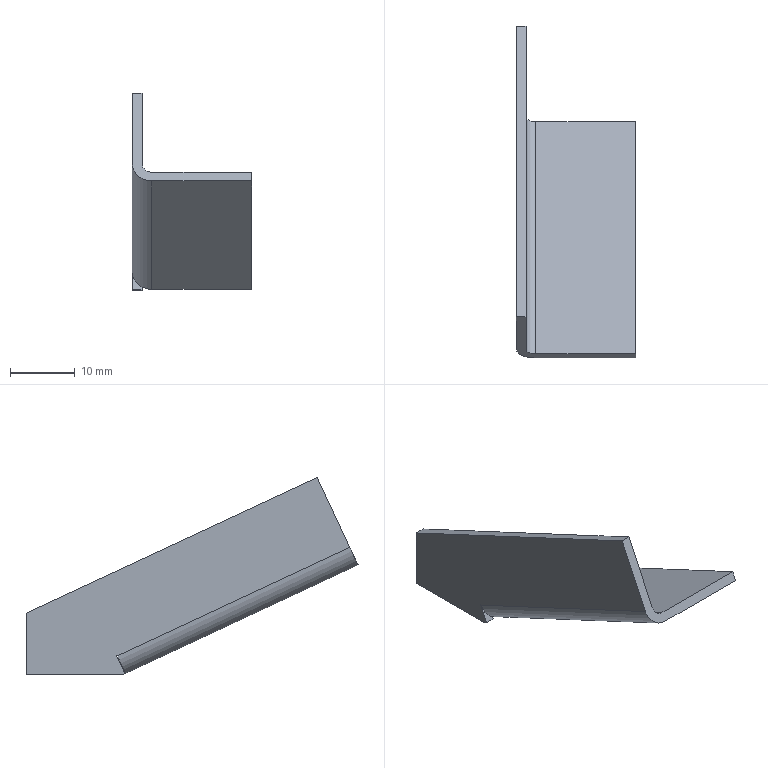Part | NX | features solid 2 | 1 solid | 15 faces | box 18.5 x 51.479 x 30.607 mm | volume 2077 mm3 | plane 13 | cylinder 2 | commonest cylinder face diameters 3 x1 6 x1
STEP:
#1=CARTESIAN_POINT('',(1091.5,-1287.659,323.577));
#2=VERTEX_POINT('',#1);
#3=CARTESIAN_POINT('',(1091.5,-1323.711,340.388));
#4=VERTEX_POINT('',#3);
#5=CARTESIAN_POINT('',(1091.5,-1287.659,323.577));
#6=DIRECTION('',(0.,-0.9063,0.4226));
#7=VECTOR('',#6,1000.);
#8=LINE('',#5,#7);
#9=EDGE_CURVE('',#2,#4,#8,.T.);
#10=ORIENTED_EDGE('',*,*,#9,.T.);
#11=CARTESIAN_POINT('',(1093.,-1324.345,339.028));
#12=VERTEX_POINT('',#11);
#13=CARTESIAN_POINT('',(1093.,-1323.711,340.388));
#14=DIRECTION('',(0.,-0.9063,0.4226));
#15=DIRECTION('',(0.,-0.4226,-0.9063));
#16=AXIS2_PLACEMENT_3D('',#13,#14,#15);
#17=CIRCLE('',#16,1.5);
#18=EDGE_CURVE('',#4,#12,#17,.T.);
#19=ORIENTED_EDGE('',*,*,#18,.T.);
#20=CARTESIAN_POINT('',(1093.,-1288.293,322.217));
#21=VERTEX_POINT('',#20);
#22=CARTESIAN_POINT('',(1093.,-1324.345,339.028));
#23=DIRECTION('',(0.,0.9063,-0.4226));
#24=VECTOR('',#23,1000.);
#25=LINE('',#22,#24);
#26=EDGE_CURVE('',#12,#21,#25,.T.);
#27=ORIENTED_EDGE('',*,*,#26,.T.);
#28=CARTESIAN_POINT('',(1093.,-1287.659,323.577));
#29=DIRECTION('',(0.,0.9063,-0.4226));
#30=DIRECTION('',(0.,-0.4226,-0.9063));
#31=AXIS2_PLACEMENT_3D('',#28,#29,#30);
#32=CIRCLE('',#31,1.5);
#33=EDGE_CURVE('',#21,#2,#32,.T.);
#34=ORIENTED_EDGE('',*,*,#33,.T.);
#35=EDGE_LOOP('',(#10,#19,#27,#34));
#36=FACE_BOUND('',#35,.T.);
#37=CARTESIAN_POINT('',(1093.,-1287.659,323.577));
#38=DIRECTION('',(0.,-0.9063,0.4226));
#39=DIRECTION('',(1.,0.,0.));
#40=AXIS2_PLACEMENT_3D('',#37,#38,#39);
#41=CYLINDRICAL_SURFACE('',#40,1.5);
#42=ADVANCED_FACE('',(#36),#41,.F.);
#43=CARTESIAN_POINT('',(1090.,-1287.659,323.577));
#44=VERTEX_POINT('',#43);
#45=CARTESIAN_POINT('',(1090.,-1323.711,340.388));
#46=VERTEX_POINT('',#45);
#47=CARTESIAN_POINT('',(1090.,-1287.659,323.577));
#48=DIRECTION('',(0.,-0.9063,0.4226));
#49=VECTOR('',#48,1000.);
#50=LINE('',#47,#49);
#51=EDGE_CURVE('',#44,#46,#50,.T.);
#52=ORIENTED_EDGE('',*,*,#51,.F.);
#53=CARTESIAN_POINT('',(1093.,-1288.927,320.858));
#54=VERTEX_POINT('',#53);
#55=CARTESIAN_POINT('',(1093.,-1287.659,323.577));
#56=DIRECTION('',(0.,0.9063,-0.4226));
#57=DIRECTION('',(1.,0.,0.));
#58=AXIS2_PLACEMENT_3D('',#55,#56,#57);
#59=CIRCLE('',#58,3.);
#60=EDGE_CURVE('',#54,#44,#59,.T.);
#61=ORIENTED_EDGE('',*,*,#60,.F.);
#62=CARTESIAN_POINT('',(1093.,-1324.979,337.669));
#63=VERTEX_POINT('',#62);
#64=CARTESIAN_POINT('',(1093.,-1324.979,337.669));
#65=DIRECTION('',(0.,0.9063,-0.4226));
#66=VECTOR('',#65,1000.);
#67=LINE('',#64,#66);
#68=EDGE_CURVE('',#63,#54,#67,.T.);
#69=ORIENTED_EDGE('',*,*,#68,.F.);
#70=CARTESIAN_POINT('',(1093.,-1323.711,340.388));
#71=DIRECTION('',(0.,-0.9063,0.4226));
#72=DIRECTION('',(1.,0.,0.));
#73=AXIS2_PLACEMENT_3D('',#70,#71,#72);
#74=CIRCLE('',#73,3.);
#75=EDGE_CURVE('',#46,#63,#74,.T.);
#76=ORIENTED_EDGE('',*,*,#75,.F.);
#77=EDGE_LOOP('',(#52,#61,#69,#76));
#78=FACE_BOUND('',#77,.T.);
#79=CARTESIAN_POINT('',(1093.,-1287.659,323.577));
#80=DIRECTION('',(0.,-0.9063,0.4226));
#81=DIRECTION('',(1.,0.,0.));
#82=AXIS2_PLACEMENT_3D('',#79,#80,#81);
#83=CYLINDRICAL_SURFACE('',#82,3.);
#84=ADVANCED_FACE('',(#78),#83,.T.);
#85=CARTESIAN_POINT('',(1108.5,-1288.293,322.217));
#86=VERTEX_POINT('',#85);
#87=CARTESIAN_POINT('',(1108.5,-1324.345,339.028));
#88=VERTEX_POINT('',#87);
#89=CARTESIAN_POINT('',(1108.5,-1288.293,322.217));
#90=DIRECTION('',(0.,-0.9063,0.4226));
#91=VECTOR('',#90,1000.);
#92=LINE('',#89,#91);
#93=EDGE_CURVE('',#86,#88,#92,.T.);
#94=ORIENTED_EDGE('',*,*,#93,.T.);
#95=CARTESIAN_POINT('',(1108.5,-1324.979,337.669));
#96=VERTEX_POINT('',#95);
#97=CARTESIAN_POINT('',(1108.5,-1324.979,337.669));
#98=DIRECTION('',(0.,0.4226,0.9063));
#99=VECTOR('',#98,1000.);
#100=LINE('',#97,#99);
#101=EDGE_CURVE('',#96,#88,#100,.T.);
#102=ORIENTED_EDGE('',*,*,#101,.F.);
#103=CARTESIAN_POINT('',(1108.5,-1288.927,320.858));
#104=VERTEX_POINT('',#103);
#105=CARTESIAN_POINT('',(1108.5,-1288.927,320.858));
#106=DIRECTION('',(0.,-0.9063,0.4226));
#107=VECTOR('',#106,1000.);
#108=LINE('',#105,#107);
#109=EDGE_CURVE('',#104,#96,#108,.T.);
#110=ORIENTED_EDGE('',*,*,#109,.F.);
#111=CARTESIAN_POINT('',(1108.5,-1288.927,320.858));
#112=DIRECTION('',(0.,0.4226,0.9063));
#113=VECTOR('',#112,1000.);
#114=LINE('',#111,#113);
#115=EDGE_CURVE('',#104,#86,#114,.T.);
#116=ORIENTED_EDGE('',*,*,#115,.T.);
#117=EDGE_LOOP('',(#94,#102,#110,#116));
#118=FACE_BOUND('',#117,.T.);
#119=CARTESIAN_POINT('',(1108.5,-1288.927,320.858));
#120=DIRECTION('',(-1.,0.,0.));
#121=DIRECTION('',(0.,0.,1.));
#122=AXIS2_PLACEMENT_3D('',#119,#120,#121);
#123=PLANE('',#122);
#124=ADVANCED_FACE('',(#118),#123,.F.);
#125=ORIENTED_EDGE('',*,*,#26,.F.);
#126=CARTESIAN_POINT('',(1091.292,-1324.345,339.028));
#127=DIRECTION('',(-1.,0.,0.));
#128=VECTOR('',#127,1000.);
#129=LINE('',#126,#128);
#130=EDGE_CURVE('',#88,#12,#129,.T.);
#131=ORIENTED_EDGE('',*,*,#130,.F.);
#132=ORIENTED_EDGE('',*,*,#93,.F.);
#133=CARTESIAN_POINT('',(1091.292,-1288.293,322.217));
#134=DIRECTION('',(1.,0.,0.));
#135=VECTOR('',#134,1000.);
#136=LINE('',#133,#135);
#137=EDGE_CURVE('',#21,#86,#136,.T.);
#138=ORIENTED_EDGE('',*,*,#137,.F.);
#139=EDGE_LOOP('',(#125,#131,#132,#138));
#140=FACE_BOUND('',#139,.T.);
#141=CARTESIAN_POINT('',(1110.,-1092.528,230.93));
#142=DIRECTION('',(0.,-0.4226,-0.9063));
#143=DIRECTION('',(0.,-0.9063,0.4226));
#144=AXIS2_PLACEMENT_3D('',#141,#142,#143);
#145=PLANE('',#144);
#146=ADVANCED_FACE('',(#140),#145,.F.);
#147=CARTESIAN_POINT('',(1091.292,-1324.979,337.669));
#148=DIRECTION('',(-1.,0.,0.));
#149=VECTOR('',#148,1000.);
#150=LINE('',#147,#149);
#151=EDGE_CURVE('',#96,#63,#150,.T.);
#152=ORIENTED_EDGE('',*,*,#151,.T.);
#153=ORIENTED_EDGE('',*,*,#68,.T.);
#154=CARTESIAN_POINT('',(1091.292,-1288.927,320.858));
#155=DIRECTION('',(1.,0.,0.));
#156=VECTOR('',#155,1000.);
#157=LINE('',#154,#156);
#158=EDGE_CURVE('',#54,#104,#157,.T.);
#159=ORIENTED_EDGE('',*,*,#158,.T.);
#160=ORIENTED_EDGE('',*,*,#109,.T.);
#161=EDGE_LOOP('',(#152,#153,#159,#160));
#162=FACE_BOUND('',#161,.T.);
#163=CARTESIAN_POINT('',(1110.,-1093.162,229.571));
#164=DIRECTION('',(0.,-0.4226,-0.9063));
#165=DIRECTION('',(0.,-0.9063,0.4226));
#166=AXIS2_PLACEMENT_3D('',#163,#164,#165);
#167=PLANE('',#166);
#168=ADVANCED_FACE('',(#162),#167,.T.);
#169=CARTESIAN_POINT('',(1091.5,-1287.617,323.667));
#170=VERTEX_POINT('',#169);
#171=CARTESIAN_POINT('',(1091.5,-1287.526,323.625));
#172=VERTEX_POINT('',#171);
#173=CARTESIAN_POINT('',(1091.5,-1287.526,323.625));
#174=DIRECTION('',(0.,0.9063,-0.4226));
#175=VECTOR('',#174,1000.);
#176=LINE('',#173,#175);
#177=EDGE_CURVE('',#170,#172,#176,.T.);
#178=ORIENTED_EDGE('',*,*,#177,.F.);
#179=CARTESIAN_POINT('',(1090.,-1287.617,323.667));
#180=VERTEX_POINT('',#179);
#181=CARTESIAN_POINT('',(1090.,-1287.617,323.667));
#182=DIRECTION('',(-1.,0.,0.));
#183=VECTOR('',#182,1000.);
#184=LINE('',#181,#183);
#185=EDGE_CURVE('',#170,#180,#184,.T.);
#186=ORIENTED_EDGE('',*,*,#185,.T.);
#187=CARTESIAN_POINT('',(1090.,-1287.526,323.625));
#188=VERTEX_POINT('',#187);
#189=CARTESIAN_POINT('',(1090.,-1287.526,323.625));
#190=DIRECTION('',(0.,0.9063,-0.4226));
#191=VECTOR('',#190,1000.);
#192=LINE('',#189,#191);
#193=EDGE_CURVE('',#180,#188,#192,.T.);
#194=ORIENTED_EDGE('',*,*,#193,.T.);
#195=CARTESIAN_POINT('',(1090.,-1287.526,323.625));
#196=DIRECTION('',(-1.,0.,0.));
#197=VECTOR('',#196,1000.);
#198=LINE('',#195,#197);
#199=EDGE_CURVE('',#172,#188,#198,.T.);
#200=ORIENTED_EDGE('',*,*,#199,.F.);
#201=EDGE_LOOP('',(#178,#186,#194,#200));
#202=FACE_BOUND('',#201,.T.);
#203=CARTESIAN_POINT('',(1090.,-1287.526,323.625));
#204=DIRECTION('',(0.,0.4226,0.9063));
#205=DIRECTION('',(1.,0.,0.));
#206=AXIS2_PLACEMENT_3D('',#203,#204,#205);
#207=PLANE('',#206);
#208=ADVANCED_FACE('',(#202),#207,.F.);
#209=ORIENTED_EDGE('',*,*,#199,.T.);
#210=CARTESIAN_POINT('',(1090.,-1288.836,320.815));
#211=VERTEX_POINT('',#210);
#212=CARTESIAN_POINT('',(1090.,-1288.836,320.815));
#213=DIRECTION('',(0.,-0.4226,-0.9063));
#214=VECTOR('',#213,1000.);
#215=LINE('',#212,#214);
#216=EDGE_CURVE('',#188,#211,#215,.T.);
#217=ORIENTED_EDGE('',*,*,#216,.T.);
#218=CARTESIAN_POINT('',(1091.5,-1288.836,320.815));
#219=VERTEX_POINT('',#218);
#220=CARTESIAN_POINT('',(1090.,-1288.836,320.815));
#221=DIRECTION('',(-1.,0.,0.));
#222=VECTOR('',#221,1000.);
#223=LINE('',#220,#222);
#224=EDGE_CURVE('',#219,#211,#223,.T.);
#225=ORIENTED_EDGE('',*,*,#224,.F.);
#226=CARTESIAN_POINT('',(1091.5,-1288.836,320.815));
#227=DIRECTION('',(0.,-0.4226,-0.9063));
#228=VECTOR('',#227,1000.);
#229=LINE('',#226,#228);
#230=EDGE_CURVE('',#172,#219,#229,.T.);
#231=ORIENTED_EDGE('',*,*,#230,.F.);
#232=EDGE_LOOP('',(#209,#217,#225,#231));
#233=FACE_BOUND('',#232,.T.);
#234=CARTESIAN_POINT('',(1090.,-1288.836,320.815));
#235=DIRECTION('',(0.,0.9063,-0.4226));
#236=DIRECTION('',(-1.,0.,0.));
#237=AXIS2_PLACEMENT_3D('',#234,#235,#236);
#238=PLANE('',#237);
#239=ADVANCED_FACE('',(#233),#238,.F.);
#240=ORIENTED_EDGE('',*,*,#9,.F.);
#241=CARTESIAN_POINT('',(1091.5,-1288.927,320.858));
#242=DIRECTION('',(0.,0.4226,0.9063));
#243=VECTOR('',#242,1000.);
#244=LINE('',#241,#243);
#245=EDGE_CURVE('',#2,#170,#244,.T.);
#246=ORIENTED_EDGE('',*,*,#245,.T.);
#247=ORIENTED_EDGE('',*,*,#177,.T.);
#248=ORIENTED_EDGE('',*,*,#230,.T.);
#249=CARTESIAN_POINT('',(1091.5,-1288.496,320.657));
#250=VERTEX_POINT('',#249);
#251=CARTESIAN_POINT('',(1091.5,-1324.979,337.669));
#252=DIRECTION('',(0.,0.9063,-0.4226));
#253=VECTOR('',#252,1000.);
#254=LINE('',#251,#253);
#255=EDGE_CURVE('',#219,#250,#254,.T.);
#256=ORIENTED_EDGE('',*,*,#255,.T.);
#257=CARTESIAN_POINT('',(1091.5,-1273.5,320.657));
#258=VERTEX_POINT('',#257);
#259=CARTESIAN_POINT('',(1091.5,-1288.496,320.657));
#260=DIRECTION('',(0.,1.,0.));
#261=VECTOR('',#260,1000.);
#262=LINE('',#259,#261);
#263=EDGE_CURVE('',#250,#258,#262,.T.);
#264=ORIENTED_EDGE('',*,*,#263,.T.);
#265=CARTESIAN_POINT('',(1091.5,-1273.5,330.215));
#266=VERTEX_POINT('',#265);
#267=CARTESIAN_POINT('',(1091.5,-1273.5,320.657));
#268=DIRECTION('',(0.,0.,1.));
#269=VECTOR('',#268,1000.);
#270=LINE('',#267,#269);
#271=EDGE_CURVE('',#258,#266,#270,.T.);
#272=ORIENTED_EDGE('',*,*,#271,.T.);
#273=CARTESIAN_POINT('',(1091.5,-1318.64,351.264));
#274=VERTEX_POINT('',#273);
#275=CARTESIAN_POINT('',(1091.5,-1273.5,330.215));
#276=DIRECTION('',(0.,-0.9063,0.4226));
#277=VECTOR('',#276,1000.);
#278=LINE('',#275,#277);
#279=EDGE_CURVE('',#266,#274,#278,.T.);
#280=ORIENTED_EDGE('',*,*,#279,.T.);
#281=CARTESIAN_POINT('',(1091.5,-1324.979,337.669));
#282=DIRECTION('',(0.,-0.4226,-0.9063));
#283=VECTOR('',#282,1000.);
#284=LINE('',#281,#283);
#285=EDGE_CURVE('',#274,#4,#284,.T.);
#286=ORIENTED_EDGE('',*,*,#285,.T.);
#287=EDGE_LOOP('',(#240,#246,#247,#248,#256,#264,#272,#280,#286));
#288=FACE_BOUND('',#287,.T.);
#289=CARTESIAN_POINT('',(1091.5,-848.5,754.25));
#290=DIRECTION('',(-1.,0.,0.));
#291=DIRECTION('',(0.,0.,1.));
#292=AXIS2_PLACEMENT_3D('',#289,#290,#291);
#293=PLANE('',#292);
#294=ADVANCED_FACE('',(#288),#293,.F.);
#295=CARTESIAN_POINT('',(1090.,-1273.5,330.215));
#296=VERTEX_POINT('',#295);
#297=CARTESIAN_POINT('',(1090.,-1318.64,351.264));
#298=VERTEX_POINT('',#297);
#299=CARTESIAN_POINT('',(1090.,-1273.5,330.215));
#300=DIRECTION('',(0.,-0.9063,0.4226));
#301=VECTOR('',#300,1000.);
#302=LINE('',#299,#301);
#303=EDGE_CURVE('',#296,#298,#302,.T.);
#304=ORIENTED_EDGE('',*,*,#303,.T.);
#305=CARTESIAN_POINT('',(1091.5,-1318.64,351.264));
#306=DIRECTION('',(-1.,0.,0.));
#307=VECTOR('',#306,1000.);
#308=LINE('',#305,#307);
#309=EDGE_CURVE('',#274,#298,#308,.T.);
#310=ORIENTED_EDGE('',*,*,#309,.F.);
#311=ORIENTED_EDGE('',*,*,#279,.F.);
#312=CARTESIAN_POINT('',(1091.5,-1273.5,330.215));
#313=DIRECTION('',(-1.,0.,0.));
#314=VECTOR('',#313,1000.);
#315=LINE('',#312,#314);
#316=EDGE_CURVE('',#266,#296,#315,.T.);
#317=ORIENTED_EDGE('',*,*,#316,.T.);
#318=EDGE_LOOP('',(#304,#310,#311,#317));
#319=FACE_BOUND('',#318,.T.);
#320=CARTESIAN_POINT('',(1091.5,-1273.5,330.215));
#321=DIRECTION('',(0.,-0.4226,-0.9063));
#322=DIRECTION('',(0.,-0.9063,0.4226));
#323=AXIS2_PLACEMENT_3D('',#320,#321,#322);
#324=PLANE('',#323);
#325=ADVANCED_FACE('',(#319),#324,.F.);
#326=CARTESIAN_POINT('',(1090.,-1273.5,320.657));
#327=VERTEX_POINT('',#326);
#328=CARTESIAN_POINT('',(1090.,-1273.5,320.657));
#329=DIRECTION('',(0.,0.,1.));
#330=VECTOR('',#329,1000.);
#331=LINE('',#328,#330);
#332=EDGE_CURVE('',#327,#296,#331,.T.);
#333=ORIENTED_EDGE('',*,*,#332,.T.);
#334=ORIENTED_EDGE('',*,*,#316,.F.);
#335=ORIENTED_EDGE('',*,*,#271,.F.);
#336=CARTESIAN_POINT('',(1091.5,-1273.5,320.657));
#337=DIRECTION('',(-1.,0.,0.));
#338=VECTOR('',#337,1000.);
#339=LINE('',#336,#338);
#340=EDGE_CURVE('',#258,#327,#339,.T.);
#341=ORIENTED_EDGE('',*,*,#340,.T.);
#342=EDGE_LOOP('',(#333,#334,#335,#341));
#343=FACE_BOUND('',#342,.T.);
#344=CARTESIAN_POINT('',(1091.5,-1273.5,320.657));
#345=DIRECTION('',(0.,-1.,0.));
#346=DIRECTION('',(0.,0.,-1.));
#347=AXIS2_PLACEMENT_3D('',#344,#345,#346);
#348=PLANE('',#347);
#349=ADVANCED_FACE('',(#343),#348,.F.);
#350=CARTESIAN_POINT('',(1090.,-1288.496,320.657));
#351=VERTEX_POINT('',#350);
#352=CARTESIAN_POINT('',(1090.,-1288.496,320.657));
#353=DIRECTION('',(0.,1.,0.));
#354=VECTOR('',#353,1000.);
#355=LINE('',#352,#354);
#356=EDGE_CURVE('',#351,#327,#355,.T.);
#357=ORIENTED_EDGE('',*,*,#356,.T.);
#358=ORIENTED_EDGE('',*,*,#340,.F.);
#359=ORIENTED_EDGE('',*,*,#263,.F.);
#360=CARTESIAN_POINT('',(1091.5,-1288.496,320.657));
#361=DIRECTION('',(-1.,0.,0.));
#362=VECTOR('',#361,1000.);
#363=LINE('',#360,#362);
#364=EDGE_CURVE('',#250,#351,#363,.T.);
#365=ORIENTED_EDGE('',*,*,#364,.T.);
#366=EDGE_LOOP('',(#357,#358,#359,#365));
#367=FACE_BOUND('',#366,.T.);
#368=CARTESIAN_POINT('',(1091.5,-1288.496,320.657));
#369=DIRECTION('',(0.,0.,1.));
#370=DIRECTION('',(1.,0.,0.));
#371=AXIS2_PLACEMENT_3D('',#368,#369,#370);
#372=PLANE('',#371);
#373=ADVANCED_FACE('',(#367),#372,.F.);
#374=ORIENTED_EDGE('',*,*,#255,.F.);
#375=ORIENTED_EDGE('',*,*,#224,.T.);
#376=CARTESIAN_POINT('',(1090.,-1324.979,337.669));
#377=DIRECTION('',(0.,0.9063,-0.4226));
#378=VECTOR('',#377,1000.);
#379=LINE('',#376,#378);
#380=EDGE_CURVE('',#211,#351,#379,.T.);
#381=ORIENTED_EDGE('',*,*,#380,.T.);
#382=ORIENTED_EDGE('',*,*,#364,.F.);
#383=EDGE_LOOP('',(#374,#375,#381,#382));
#384=FACE_BOUND('',#383,.T.);
#385=CARTESIAN_POINT('',(1091.5,-1324.979,337.669));
#386=DIRECTION('',(0.,0.4226,0.9063));
#387=DIRECTION('',(1.,0.,0.));
#388=AXIS2_PLACEMENT_3D('',#385,#386,#387);
#389=PLANE('',#388);
#390=ADVANCED_FACE('',(#384),#389,.F.);
#391=CARTESIAN_POINT('',(1090.,-1288.927,320.858));
#392=DIRECTION('',(0.,0.4226,0.9063));
#393=VECTOR('',#392,1000.);
#394=LINE('',#391,#393);
#395=EDGE_CURVE('',#44,#180,#394,.T.);
#396=ORIENTED_EDGE('',*,*,#395,.F.);
#397=ORIENTED_EDGE('',*,*,#51,.T.);
#398=CARTESIAN_POINT('',(1090.,-1324.979,337.669));
#399=DIRECTION('',(0.,-0.4226,-0.9063));
#400=VECTOR('',#399,1000.);
#401=LINE('',#398,#400);
#402=EDGE_CURVE('',#298,#46,#401,.T.);
#403=ORIENTED_EDGE('',*,*,#402,.F.);
#404=ORIENTED_EDGE('',*,*,#303,.F.);
#405=ORIENTED_EDGE('',*,*,#332,.F.);
#406=ORIENTED_EDGE('',*,*,#356,.F.);
#407=ORIENTED_EDGE('',*,*,#380,.F.);
#408=ORIENTED_EDGE('',*,*,#216,.F.);
#409=ORIENTED_EDGE('',*,*,#193,.F.);
#410=EDGE_LOOP('',(#396,#397,#403,#404,#405,#406,#407,#408,#409));
#411=FACE_BOUND('',#410,.T.);
#412=CARTESIAN_POINT('',(1090.,-848.5,754.25));
#413=DIRECTION('',(-1.,0.,0.));
#414=DIRECTION('',(0.,0.,1.));
#415=AXIS2_PLACEMENT_3D('',#412,#413,#414);
#416=PLANE('',#415);
#417=ADVANCED_FACE('',(#411),#416,.T.);
#418=ORIENTED_EDGE('',*,*,#245,.F.);
#419=ORIENTED_EDGE('',*,*,#33,.F.);
#420=ORIENTED_EDGE('',*,*,#137,.T.);
#421=ORIENTED_EDGE('',*,*,#115,.F.);
#422=ORIENTED_EDGE('',*,*,#158,.F.);
#423=ORIENTED_EDGE('',*,*,#60,.T.);
#424=ORIENTED_EDGE('',*,*,#395,.T.);
#425=ORIENTED_EDGE('',*,*,#185,.F.);
#426=EDGE_LOOP('',(#418,#419,#420,#421,#422,#423,#424,#425));
#427=FACE_BOUND('',#426,.T.);
#428=CARTESIAN_POINT('',(1090.,-1288.927,320.858));
#429=DIRECTION('',(0.,-0.9063,0.4226));
#430=DIRECTION('',(-1.,0.,0.));
#431=AXIS2_PLACEMENT_3D('',#428,#429,#430);
#432=PLANE('',#431);
#433=ADVANCED_FACE('',(#427),#432,.F.);
#434=ORIENTED_EDGE('',*,*,#402,.T.);
#435=ORIENTED_EDGE('',*,*,#75,.T.);
#436=ORIENTED_EDGE('',*,*,#151,.F.);
#437=ORIENTED_EDGE('',*,*,#101,.T.);
#438=ORIENTED_EDGE('',*,*,#130,.T.);
#439=ORIENTED_EDGE('',*,*,#18,.F.);
#440=ORIENTED_EDGE('',*,*,#285,.F.);
#441=ORIENTED_EDGE('',*,*,#309,.T.);
#442=EDGE_LOOP('',(#434,#435,#436,#437,#438,#439,#440,#441));
#443=FACE_BOUND('',#442,.T.);
#444=CARTESIAN_POINT('',(1091.5,-1324.979,337.669));
#445=DIRECTION('',(0.,0.9063,-0.4226));
#446=DIRECTION('',(-1.,0.,0.));
#447=AXIS2_PLACEMENT_3D('',#444,#445,#446);
#448=PLANE('',#447);
#449=ADVANCED_FACE('',(#443),#448,.F.);
#450=CLOSED_SHELL('',(#42,#84,#124,#146,#168,#208,#239,#294,#325,#349,#373,#390,#417,#433,#449));
#451=MANIFOLD_SOLID_BREP('',#450);
#452=(LENGTH_UNIT()NAMED_UNIT(*)SI_UNIT(.MILLI.,.METRE.));
#453=UNCERTAINTY_MEASURE_WITH_UNIT(LENGTH_MEASURE(0.00001),#452,'','');
#454=(NAMED_UNIT(*)PLANE_ANGLE_UNIT()SI_UNIT($,.RADIAN.));
#455=(NAMED_UNIT(*)SI_UNIT($,.STERADIAN.)SOLID_ANGLE_UNIT());
#456=(GEOMETRIC_REPRESENTATION_CONTEXT(3)GLOBAL_UNCERTAINTY_ASSIGNED_CONTEXT((#453))GLOBAL_UNIT_ASSIGNED_CONTEXT((#452,#454,#455))REPRESENTATION_CONTEXT('',''));
#457=ADVANCED_BREP_SHAPE_REPRESENTATION('',(#451),#456);